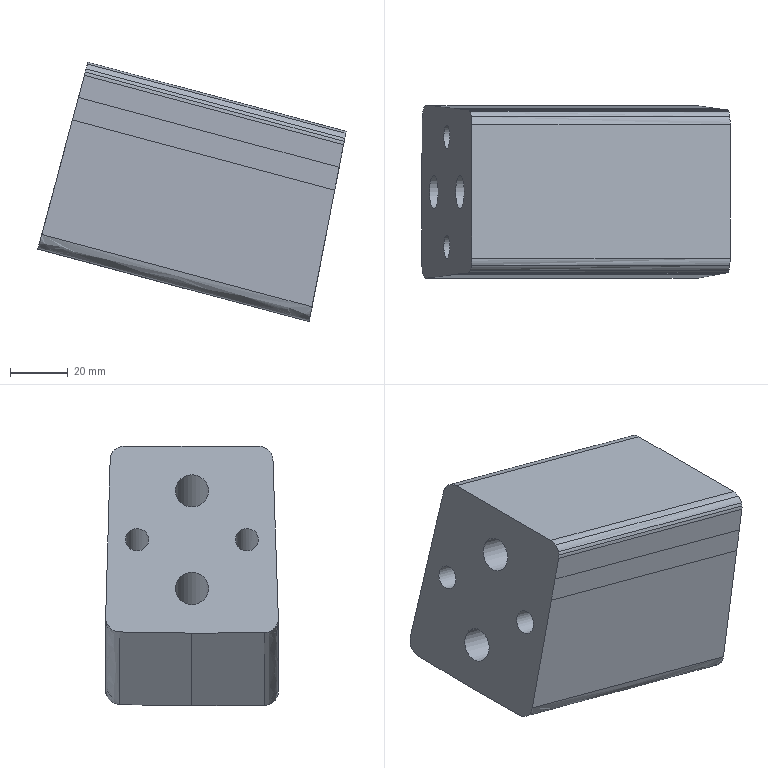Part | NX | features solid 2 | 1 solid | 39 faces | box 106.599 x 59.709 x 89.775 mm | volume 329029 mm3 | spline 22 | plane 9 | cylinder 8 | commonest cylinder face diameters 5.1 x2 8 x2 11.507 x2 18.008 x2